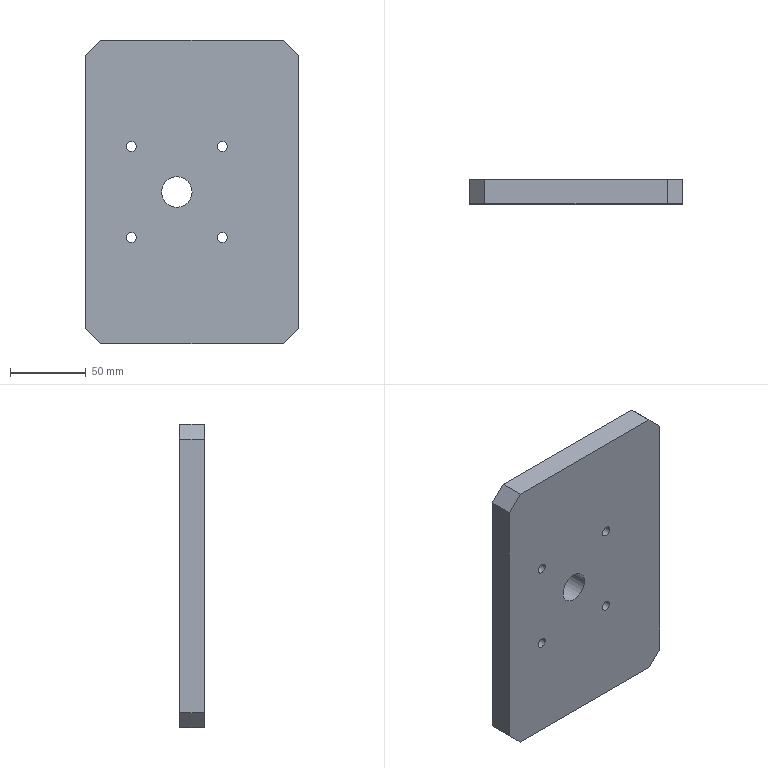Part | STEP file | M6 六角头Screw的柱形沉头Hole 2 | 1 solid | 32 faces | box 140 x 16 x 200 mm | volume 435392 mm3 | cylinder 18 | plane 14 | commonest cylinder face diameters 6.6 x8 14.55 x8 20 x2
STEP:
#1=CARTESIAN_POINT('',(-1451.463,1675.114,2786.751));
#2=VERTEX_POINT('',#1);
#3=CARTESIAN_POINT('',(-1466.013,1675.114,2786.751));
#4=VERTEX_POINT('',#3);
#5=CARTESIAN_POINT('',(-1458.738,1675.114,2786.751));
#6=DIRECTION('',(0.,1.,0.));
#7=DIRECTION('',(-1.,0.,0.));
#8=AXIS2_PLACEMENT_3D('',#5,#6,#7);
#9=CIRCLE('',#8,7.275);
#10=EDGE_CURVE('',#2,#4,#9,.T.);
#11=ORIENTED_EDGE('',*,*,#10,.F.);
#12=CARTESIAN_POINT('',(-1451.463,1679.264,2786.751));
#13=VERTEX_POINT('',#12);
#14=CARTESIAN_POINT('',(-1451.463,1679.264,2786.751));
#15=DIRECTION('',(0.,1.,0.));
#16=VECTOR('',#15,1000.);
#17=LINE('',#14,#16);
#18=EDGE_CURVE('',#2,#13,#17,.T.);
#19=ORIENTED_EDGE('',*,*,#18,.T.);
#20=CARTESIAN_POINT('',(-1466.013,1679.264,2786.751));
#21=VERTEX_POINT('',#20);
#22=CARTESIAN_POINT('',(-1458.738,1679.264,2786.751));
#23=DIRECTION('',(0.,1.,0.));
#24=DIRECTION('',(-1.,0.,0.));
#25=AXIS2_PLACEMENT_3D('',#22,#23,#24);
#26=CIRCLE('',#25,7.275);
#27=EDGE_CURVE('',#13,#21,#26,.T.);
#28=ORIENTED_EDGE('',*,*,#27,.T.);
#29=CARTESIAN_POINT('',(-1466.013,1679.264,2786.751));
#30=DIRECTION('',(0.,1.,0.));
#31=VECTOR('',#30,1000.);
#32=LINE('',#29,#31);
#33=EDGE_CURVE('',#4,#21,#32,.T.);
#34=ORIENTED_EDGE('',*,*,#33,.F.);
#35=EDGE_LOOP('',(#11,#19,#28,#34));
#36=FACE_OUTER_BOUND('',#35,.T.);
#37=CARTESIAN_POINT('',(-1458.738,1679.264,2786.751));
#38=DIRECTION('',(0.,1.,0.));
#39=DIRECTION('',(1.,0.,0.));
#40=AXIS2_PLACEMENT_3D('',#37,#38,#39);
#41=CYLINDRICAL_SURFACE('',#40,7.275);
#42=ADVANCED_FACE('',(#36),#41,.F.);
#43=CARTESIAN_POINT('',(-1455.438,1663.264,2786.751));
#44=VERTEX_POINT('',#43);
#45=CARTESIAN_POINT('',(-1462.038,1663.264,2786.751));
#46=VERTEX_POINT('',#45);
#47=CARTESIAN_POINT('',(-1458.738,1663.264,2786.751));
#48=DIRECTION('',(0.,1.,0.));
#49=DIRECTION('',(-1.,0.,0.));
#50=AXIS2_PLACEMENT_3D('',#47,#48,#49);
#51=CIRCLE('',#50,3.3);
#52=EDGE_CURVE('',#44,#46,#51,.T.);
#53=ORIENTED_EDGE('',*,*,#52,.F.);
#54=CARTESIAN_POINT('',(-1455.438,1675.114,2786.751));
#55=VERTEX_POINT('',#54);
#56=CARTESIAN_POINT('',(-1455.438,1679.264,2786.751));
#57=DIRECTION('',(0.,1.,0.));
#58=VECTOR('',#57,1000.);
#59=LINE('',#56,#58);
#60=EDGE_CURVE('',#44,#55,#59,.T.);
#61=ORIENTED_EDGE('',*,*,#60,.T.);
#62=CARTESIAN_POINT('',(-1462.038,1675.114,2786.751));
#63=VERTEX_POINT('',#62);
#64=CARTESIAN_POINT('',(-1458.738,1675.114,2786.751));
#65=DIRECTION('',(0.,1.,0.));
#66=DIRECTION('',(-1.,0.,0.));
#67=AXIS2_PLACEMENT_3D('',#64,#65,#66);
#68=CIRCLE('',#67,3.3);
#69=EDGE_CURVE('',#55,#63,#68,.T.);
#70=ORIENTED_EDGE('',*,*,#69,.T.);
#71=CARTESIAN_POINT('',(-1462.038,1679.264,2786.751));
#72=DIRECTION('',(0.,1.,0.));
#73=VECTOR('',#72,1000.);
#74=LINE('',#71,#73);
#75=EDGE_CURVE('',#46,#63,#74,.T.);
#76=ORIENTED_EDGE('',*,*,#75,.F.);
#77=EDGE_LOOP('',(#53,#61,#70,#76));
#78=FACE_OUTER_BOUND('',#77,.T.);
#79=CARTESIAN_POINT('',(-1458.738,1679.264,2786.751));
#80=DIRECTION('',(0.,1.,0.));
#81=DIRECTION('',(1.,0.,0.));
#82=AXIS2_PLACEMENT_3D('',#79,#80,#81);
#83=CYLINDRICAL_SURFACE('',#82,3.3);
#84=ADVANCED_FACE('',(#78),#83,.F.);
#85=CARTESIAN_POINT('',(-1511.463,1675.114,2846.751));
#86=VERTEX_POINT('',#85);
#87=CARTESIAN_POINT('',(-1526.013,1675.114,2846.751));
#88=VERTEX_POINT('',#87);
#89=CARTESIAN_POINT('',(-1518.738,1675.114,2846.751));
#90=DIRECTION('',(0.,1.,0.));
#91=DIRECTION('',(-1.,0.,0.));
#92=AXIS2_PLACEMENT_3D('',#89,#90,#91);
#93=CIRCLE('',#92,7.275);
#94=EDGE_CURVE('',#86,#88,#93,.T.);
#95=ORIENTED_EDGE('',*,*,#94,.F.);
#96=CARTESIAN_POINT('',(-1511.463,1679.264,2846.751));
#97=VERTEX_POINT('',#96);
#98=CARTESIAN_POINT('',(-1511.463,1679.264,2846.751));
#99=DIRECTION('',(0.,1.,0.));
#100=VECTOR('',#99,1000.);
#101=LINE('',#98,#100);
#102=EDGE_CURVE('',#86,#97,#101,.T.);
#103=ORIENTED_EDGE('',*,*,#102,.T.);
#104=CARTESIAN_POINT('',(-1526.013,1679.264,2846.751));
#105=VERTEX_POINT('',#104);
#106=CARTESIAN_POINT('',(-1518.738,1679.264,2846.751));
#107=DIRECTION('',(0.,1.,0.));
#108=DIRECTION('',(-1.,0.,0.));
#109=AXIS2_PLACEMENT_3D('',#106,#107,#108);
#110=CIRCLE('',#109,7.275);
#111=EDGE_CURVE('',#97,#105,#110,.T.);
#112=ORIENTED_EDGE('',*,*,#111,.T.);
#113=CARTESIAN_POINT('',(-1526.013,1679.264,2846.751));
#114=DIRECTION('',(0.,1.,0.));
#115=VECTOR('',#114,1000.);
#116=LINE('',#113,#115);
#117=EDGE_CURVE('',#88,#105,#116,.T.);
#118=ORIENTED_EDGE('',*,*,#117,.F.);
#119=EDGE_LOOP('',(#95,#103,#112,#118));
#120=FACE_OUTER_BOUND('',#119,.T.);
#121=CARTESIAN_POINT('',(-1518.738,1679.264,2846.751));
#122=DIRECTION('',(0.,1.,0.));
#123=DIRECTION('',(1.,0.,0.));
#124=AXIS2_PLACEMENT_3D('',#121,#122,#123);
#125=CYLINDRICAL_SURFACE('',#124,7.275);
#126=ADVANCED_FACE('',(#120),#125,.F.);
#127=CARTESIAN_POINT('',(-1515.438,1663.264,2846.751));
#128=VERTEX_POINT('',#127);
#129=CARTESIAN_POINT('',(-1522.038,1663.264,2846.751));
#130=VERTEX_POINT('',#129);
#131=CARTESIAN_POINT('',(-1518.738,1663.264,2846.751));
#132=DIRECTION('',(0.,1.,0.));
#133=DIRECTION('',(-1.,0.,0.));
#134=AXIS2_PLACEMENT_3D('',#131,#132,#133);
#135=CIRCLE('',#134,3.3);
#136=EDGE_CURVE('',#128,#130,#135,.T.);
#137=ORIENTED_EDGE('',*,*,#136,.F.);
#138=CARTESIAN_POINT('',(-1515.438,1675.114,2846.751));
#139=VERTEX_POINT('',#138);
#140=CARTESIAN_POINT('',(-1515.438,1679.264,2846.751));
#141=DIRECTION('',(0.,1.,0.));
#142=VECTOR('',#141,1000.);
#143=LINE('',#140,#142);
#144=EDGE_CURVE('',#128,#139,#143,.T.);
#145=ORIENTED_EDGE('',*,*,#144,.T.);
#146=CARTESIAN_POINT('',(-1522.038,1675.114,2846.751));
#147=VERTEX_POINT('',#146);
#148=CARTESIAN_POINT('',(-1518.738,1675.114,2846.751));
#149=DIRECTION('',(0.,1.,0.));
#150=DIRECTION('',(-1.,0.,0.));
#151=AXIS2_PLACEMENT_3D('',#148,#149,#150);
#152=CIRCLE('',#151,3.3);
#153=EDGE_CURVE('',#139,#147,#152,.T.);
#154=ORIENTED_EDGE('',*,*,#153,.T.);
#155=CARTESIAN_POINT('',(-1522.038,1679.264,2846.751));
#156=DIRECTION('',(0.,1.,0.));
#157=VECTOR('',#156,1000.);
#158=LINE('',#155,#157);
#159=EDGE_CURVE('',#130,#147,#158,.T.);
#160=ORIENTED_EDGE('',*,*,#159,.F.);
#161=EDGE_LOOP('',(#137,#145,#154,#160));
#162=FACE_OUTER_BOUND('',#161,.T.);
#163=CARTESIAN_POINT('',(-1518.738,1679.264,2846.751));
#164=DIRECTION('',(0.,1.,0.));
#165=DIRECTION('',(1.,0.,0.));
#166=AXIS2_PLACEMENT_3D('',#163,#164,#165);
#167=CYLINDRICAL_SURFACE('',#166,3.3);
#168=ADVANCED_FACE('',(#162),#167,.F.);
#169=CARTESIAN_POINT('',(-1451.463,1675.114,2846.751));
#170=VERTEX_POINT('',#169);
#171=CARTESIAN_POINT('',(-1466.013,1675.114,2846.751));
#172=VERTEX_POINT('',#171);
#173=CARTESIAN_POINT('',(-1458.738,1675.114,2846.751));
#174=DIRECTION('',(0.,1.,0.));
#175=DIRECTION('',(-1.,0.,0.));
#176=AXIS2_PLACEMENT_3D('',#173,#174,#175);
#177=CIRCLE('',#176,7.275);
#178=EDGE_CURVE('',#170,#172,#177,.T.);
#179=ORIENTED_EDGE('',*,*,#178,.F.);
#180=CARTESIAN_POINT('',(-1451.463,1679.264,2846.751));
#181=VERTEX_POINT('',#180);
#182=CARTESIAN_POINT('',(-1451.463,1679.264,2846.751));
#183=DIRECTION('',(0.,1.,0.));
#184=VECTOR('',#183,1000.);
#185=LINE('',#182,#184);
#186=EDGE_CURVE('',#170,#181,#185,.T.);
#187=ORIENTED_EDGE('',*,*,#186,.T.);
#188=CARTESIAN_POINT('',(-1466.013,1679.264,2846.751));
#189=VERTEX_POINT('',#188);
#190=CARTESIAN_POINT('',(-1458.738,1679.264,2846.751));
#191=DIRECTION('',(0.,1.,0.));
#192=DIRECTION('',(-1.,0.,0.));
#193=AXIS2_PLACEMENT_3D('',#190,#191,#192);
#194=CIRCLE('',#193,7.275);
#195=EDGE_CURVE('',#181,#189,#194,.T.);
#196=ORIENTED_EDGE('',*,*,#195,.T.);
#197=CARTESIAN_POINT('',(-1466.013,1679.264,2846.751));
#198=DIRECTION('',(0.,1.,0.));
#199=VECTOR('',#198,1000.);
#200=LINE('',#197,#199);
#201=EDGE_CURVE('',#172,#189,#200,.T.);
#202=ORIENTED_EDGE('',*,*,#201,.F.);
#203=EDGE_LOOP('',(#179,#187,#196,#202));
#204=FACE_OUTER_BOUND('',#203,.T.);
#205=CARTESIAN_POINT('',(-1458.738,1679.264,2846.751));
#206=DIRECTION('',(0.,1.,0.));
#207=DIRECTION('',(1.,0.,0.));
#208=AXIS2_PLACEMENT_3D('',#205,#206,#207);
#209=CYLINDRICAL_SURFACE('',#208,7.275);
#210=ADVANCED_FACE('',(#204),#209,.F.);
#211=CARTESIAN_POINT('',(-1455.438,1663.264,2846.751));
#212=VERTEX_POINT('',#211);
#213=CARTESIAN_POINT('',(-1462.038,1663.264,2846.751));
#214=VERTEX_POINT('',#213);
#215=CARTESIAN_POINT('',(-1458.738,1663.264,2846.751));
#216=DIRECTION('',(0.,1.,0.));
#217=DIRECTION('',(-1.,0.,0.));
#218=AXIS2_PLACEMENT_3D('',#215,#216,#217);
#219=CIRCLE('',#218,3.3);
#220=EDGE_CURVE('',#212,#214,#219,.T.);
#221=ORIENTED_EDGE('',*,*,#220,.F.);
#222=CARTESIAN_POINT('',(-1455.438,1675.114,2846.751));
#223=VERTEX_POINT('',#222);
#224=CARTESIAN_POINT('',(-1455.438,1679.264,2846.751));
#225=DIRECTION('',(0.,1.,0.));
#226=VECTOR('',#225,1000.);
#227=LINE('',#224,#226);
#228=EDGE_CURVE('',#212,#223,#227,.T.);
#229=ORIENTED_EDGE('',*,*,#228,.T.);
#230=CARTESIAN_POINT('',(-1462.038,1675.114,2846.751));
#231=VERTEX_POINT('',#230);
#232=CARTESIAN_POINT('',(-1458.738,1675.114,2846.751));
#233=DIRECTION('',(0.,1.,0.));
#234=DIRECTION('',(-1.,0.,0.));
#235=AXIS2_PLACEMENT_3D('',#232,#233,#234);
#236=CIRCLE('',#235,3.3);
#237=EDGE_CURVE('',#223,#231,#236,.T.);
#238=ORIENTED_EDGE('',*,*,#237,.T.);
#239=CARTESIAN_POINT('',(-1462.038,1679.264,2846.751));
#240=DIRECTION('',(0.,1.,0.));
#241=VECTOR('',#240,1000.);
#242=LINE('',#239,#241);
#243=EDGE_CURVE('',#214,#231,#242,.T.);
#244=ORIENTED_EDGE('',*,*,#243,.F.);
#245=EDGE_LOOP('',(#221,#229,#238,#244));
#246=FACE_OUTER_BOUND('',#245,.T.);
#247=CARTESIAN_POINT('',(-1458.738,1679.264,2846.751));
#248=DIRECTION('',(0.,1.,0.));
#249=DIRECTION('',(1.,0.,0.));
#250=AXIS2_PLACEMENT_3D('',#247,#248,#249);
#251=CYLINDRICAL_SURFACE('',#250,3.3);
#252=ADVANCED_FACE('',(#246),#251,.F.);
#253=CARTESIAN_POINT('',(-1511.463,1675.114,2786.751));
#254=VERTEX_POINT('',#253);
#255=CARTESIAN_POINT('',(-1526.013,1675.114,2786.751));
#256=VERTEX_POINT('',#255);
#257=CARTESIAN_POINT('',(-1518.738,1675.114,2786.751));
#258=DIRECTION('',(0.,1.,0.));
#259=DIRECTION('',(-1.,0.,0.));
#260=AXIS2_PLACEMENT_3D('',#257,#258,#259);
#261=CIRCLE('',#260,7.275);
#262=EDGE_CURVE('',#254,#256,#261,.T.);
#263=ORIENTED_EDGE('',*,*,#262,.F.);
#264=CARTESIAN_POINT('',(-1511.463,1679.264,2786.751));
#265=VERTEX_POINT('',#264);
#266=CARTESIAN_POINT('',(-1511.463,1679.264,2786.751));
#267=DIRECTION('',(0.,1.,0.));
#268=VECTOR('',#267,1000.);
#269=LINE('',#266,#268);
#270=EDGE_CURVE('',#254,#265,#269,.T.);
#271=ORIENTED_EDGE('',*,*,#270,.T.);
#272=CARTESIAN_POINT('',(-1526.013,1679.264,2786.751));
#273=VERTEX_POINT('',#272);
#274=CARTESIAN_POINT('',(-1518.738,1679.264,2786.751));
#275=DIRECTION('',(0.,1.,0.));
#276=DIRECTION('',(-1.,0.,0.));
#277=AXIS2_PLACEMENT_3D('',#274,#275,#276);
#278=CIRCLE('',#277,7.275);
#279=EDGE_CURVE('',#265,#273,#278,.T.);
#280=ORIENTED_EDGE('',*,*,#279,.T.);
#281=CARTESIAN_POINT('',(-1526.013,1679.264,2786.751));
#282=DIRECTION('',(0.,1.,0.));
#283=VECTOR('',#282,1000.);
#284=LINE('',#281,#283);
#285=EDGE_CURVE('',#256,#273,#284,.T.);
#286=ORIENTED_EDGE('',*,*,#285,.F.);
#287=EDGE_LOOP('',(#263,#271,#280,#286));
#288=FACE_OUTER_BOUND('',#287,.T.);
#289=CARTESIAN_POINT('',(-1518.738,1679.264,2786.751));
#290=DIRECTION('',(0.,1.,0.));
#291=DIRECTION('',(1.,0.,0.));
#292=AXIS2_PLACEMENT_3D('',#289,#290,#291);
#293=CYLINDRICAL_SURFACE('',#292,7.275);
#294=ADVANCED_FACE('',(#288),#293,.F.);
#295=CARTESIAN_POINT('',(-1515.438,1663.264,2786.751));
#296=VERTEX_POINT('',#295);
#297=CARTESIAN_POINT('',(-1522.038,1663.264,2786.751));
#298=VERTEX_POINT('',#297);
#299=CARTESIAN_POINT('',(-1518.738,1663.264,2786.751));
#300=DIRECTION('',(0.,1.,0.));
#301=DIRECTION('',(-1.,0.,0.));
#302=AXIS2_PLACEMENT_3D('',#299,#300,#301);
#303=CIRCLE('',#302,3.3);
#304=EDGE_CURVE('',#296,#298,#303,.T.);
#305=ORIENTED_EDGE('',*,*,#304,.F.);
#306=CARTESIAN_POINT('',(-1515.438,1675.114,2786.751));
#307=VERTEX_POINT('',#306);
#308=CARTESIAN_POINT('',(-1515.438,1679.264,2786.751));
#309=DIRECTION('',(0.,1.,0.));
#310=VECTOR('',#309,1000.);
#311=LINE('',#308,#310);
#312=EDGE_CURVE('',#296,#307,#311,.T.);
#313=ORIENTED_EDGE('',*,*,#312,.T.);
#314=CARTESIAN_POINT('',(-1522.038,1675.114,2786.751));
#315=VERTEX_POINT('',#314);
#316=CARTESIAN_POINT('',(-1518.738,1675.114,2786.751));
#317=DIRECTION('',(0.,1.,0.));
#318=DIRECTION('',(-1.,0.,0.));
#319=AXIS2_PLACEMENT_3D('',#316,#317,#318);
#320=CIRCLE('',#319,3.3);
#321=EDGE_CURVE('',#307,#315,#320,.T.);
#322=ORIENTED_EDGE('',*,*,#321,.T.);
#323=CARTESIAN_POINT('',(-1522.038,1679.264,2786.751));
#324=DIRECTION('',(0.,1.,0.));
#325=VECTOR('',#324,1000.);
#326=LINE('',#323,#325);
#327=EDGE_CURVE('',#298,#315,#326,.T.);
#328=ORIENTED_EDGE('',*,*,#327,.F.);
#329=EDGE_LOOP('',(#305,#313,#322,#328));
#330=FACE_OUTER_BOUND('',#329,.T.);
#331=CARTESIAN_POINT('',(-1518.738,1679.264,2786.751));
#332=DIRECTION('',(0.,1.,0.));
#333=DIRECTION('',(1.,0.,0.));
#334=AXIS2_PLACEMENT_3D('',#331,#332,#333);
#335=CYLINDRICAL_SURFACE('',#334,3.3);
#336=ADVANCED_FACE('',(#330),#335,.F.);
#337=CARTESIAN_POINT('',(-1478.738,1663.264,2816.751));
#338=VERTEX_POINT('',#337);
#339=CARTESIAN_POINT('',(-1498.738,1663.264,2816.751));
#340=VERTEX_POINT('',#339);
#341=CARTESIAN_POINT('',(-1488.738,1663.264,2816.751));
#342=DIRECTION('',(0.,1.,0.));
#343=DIRECTION('',(-1.,0.,0.));
#344=AXIS2_PLACEMENT_3D('',#341,#342,#343);
#345=CIRCLE('',#344,10.);
#346=EDGE_CURVE('',#338,#340,#345,.T.);
#347=ORIENTED_EDGE('',*,*,#346,.F.);
#348=CARTESIAN_POINT('',(-1478.738,1679.264,2816.751));
#349=VERTEX_POINT('',#348);
#350=CARTESIAN_POINT('',(-1478.738,1573.264,2816.751));
#351=DIRECTION('',(0.,1.,0.));
#352=VECTOR('',#351,1000.);
#353=LINE('',#350,#352);
#354=EDGE_CURVE('',#338,#349,#353,.T.);
#355=ORIENTED_EDGE('',*,*,#354,.T.);
#356=CARTESIAN_POINT('',(-1498.738,1679.264,2816.751));
#357=VERTEX_POINT('',#356);
#358=CARTESIAN_POINT('',(-1488.738,1679.264,2816.751));
#359=DIRECTION('',(0.,1.,0.));
#360=DIRECTION('',(-1.,0.,0.));
#361=AXIS2_PLACEMENT_3D('',#358,#359,#360);
#362=CIRCLE('',#361,10.);
#363=EDGE_CURVE('',#349,#357,#362,.T.);
#364=ORIENTED_EDGE('',*,*,#363,.T.);
#365=CARTESIAN_POINT('',(-1498.738,1573.264,2816.751));
#366=DIRECTION('',(0.,1.,0.));
#367=VECTOR('',#366,1000.);
#368=LINE('',#365,#367);
#369=EDGE_CURVE('',#340,#357,#368,.T.);
#370=ORIENTED_EDGE('',*,*,#369,.F.);
#371=EDGE_LOOP('',(#347,#355,#364,#370));
#372=FACE_OUTER_BOUND('',#371,.T.);
#373=CARTESIAN_POINT('',(-1488.738,1573.264,2816.751));
#374=DIRECTION('',(0.,1.,0.));
#375=DIRECTION('',(1.,0.,0.));
#376=AXIS2_PLACEMENT_3D('',#373,#374,#375);
#377=CYLINDRICAL_SURFACE('',#376,10.);
#378=ADVANCED_FACE('',(#372),#377,.F.);
#379=CARTESIAN_POINT('',(-1538.738,1663.264,2916.751));
#380=VERTEX_POINT('',#379);
#381=CARTESIAN_POINT('',(-1418.738,1663.264,2916.751));
#382=VERTEX_POINT('',#381);
#383=CARTESIAN_POINT('',(-1408.738,1663.264,2916.751));
#384=DIRECTION('',(1.,0.,0.));
#385=VECTOR('',#384,1000.);
#386=LINE('',#383,#385);
#387=EDGE_CURVE('',#380,#382,#386,.T.);
#388=ORIENTED_EDGE('',*,*,#387,.T.);
#389=CARTESIAN_POINT('',(-1418.738,1679.264,2916.751));
#390=VERTEX_POINT('',#389);
#391=CARTESIAN_POINT('',(-1418.738,1679.264,2916.751));
#392=DIRECTION('',(0.,1.,0.));
#393=VECTOR('',#392,1000.);
#394=LINE('',#391,#393);
#395=EDGE_CURVE('',#382,#390,#394,.T.);
#396=ORIENTED_EDGE('',*,*,#395,.T.);
#397=CARTESIAN_POINT('',(-1538.738,1679.264,2916.751));
#398=VERTEX_POINT('',#397);
#399=CARTESIAN_POINT('',(-1408.738,1679.264,2916.751));
#400=DIRECTION('',(1.,0.,0.));
#401=VECTOR('',#400,1000.);
#402=LINE('',#399,#401);
#403=EDGE_CURVE('',#398,#390,#402,.T.);
#404=ORIENTED_EDGE('',*,*,#403,.F.);
#405=CARTESIAN_POINT('',(-1538.738,1679.264,2916.751));
#406=DIRECTION('',(0.,-1.,0.));
#407=VECTOR('',#406,1000.);
#408=LINE('',#405,#407);
#409=EDGE_CURVE('',#398,#380,#408,.T.);
#410=ORIENTED_EDGE('',*,*,#409,.T.);
#411=EDGE_LOOP('',(#388,#396,#404,#410));
#412=FACE_OUTER_BOUND('',#411,.T.);
#413=CARTESIAN_POINT('',(-1408.738,1679.264,2916.751));
#414=DIRECTION('',(0.,0.,-1.));
#415=DIRECTION('',(1.,0.,0.));
#416=AXIS2_PLACEMENT_3D('',#413,#414,#415);
#417=PLANE('',#416);
#418=ADVANCED_FACE('',(#412),#417,.F.);
#419=CARTESIAN_POINT('',(-1408.738,1679.264,2906.751));
#420=VERTEX_POINT('',#419);
#421=CARTESIAN_POINT('',(-1408.738,1679.264,2726.751));
#422=VERTEX_POINT('',#421);
#423=CARTESIAN_POINT('',(-1408.738,1679.264,2716.751));
#424=DIRECTION('',(0.,0.,-1.));
#425=VECTOR('',#424,1000.);
#426=LINE('',#423,#425);
#427=EDGE_CURVE('',#420,#422,#426,.T.);
#428=ORIENTED_EDGE('',*,*,#427,.F.);
#429=CARTESIAN_POINT('',(-1408.738,1663.264,2906.751));
#430=VERTEX_POINT('',#429);
#431=CARTESIAN_POINT('',(-1408.738,1679.264,2906.751));
#432=DIRECTION('',(0.,-1.,0.));
#433=VECTOR('',#432,1000.);
#434=LINE('',#431,#433);
#435=EDGE_CURVE('',#420,#430,#434,.T.);
#436=ORIENTED_EDGE('',*,*,#435,.T.);
#437=CARTESIAN_POINT('',(-1408.738,1663.264,2726.751));
#438=VERTEX_POINT('',#437);
#439=CARTESIAN_POINT('',(-1408.738,1663.264,2716.751));
#440=DIRECTION('',(0.,0.,-1.));
#441=VECTOR('',#440,1000.);
#442=LINE('',#439,#441);
#443=EDGE_CURVE('',#430,#438,#442,.T.);
#444=ORIENTED_EDGE('',*,*,#443,.T.);
#445=CARTESIAN_POINT('',(-1408.738,1679.264,2726.751));
#446=DIRECTION('',(0.,1.,0.));
#447=VECTOR('',#446,1000.);
#448=LINE('',#445,#447);
#449=EDGE_CURVE('',#438,#422,#448,.T.);
#450=ORIENTED_EDGE('',*,*,#449,.T.);
#451=EDGE_LOOP('',(#428,#436,#444,#450));
#452=FACE_OUTER_BOUND('',#451,.T.);
#453=CARTESIAN_POINT('',(-1408.738,1679.264,2716.751));
#454=DIRECTION('',(-1.,0.,0.));
#455=DIRECTION('',(0.,0.,-1.));
#456=AXIS2_PLACEMENT_3D('',#453,#454,#455);
#457=PLANE('',#456);
#458=ADVANCED_FACE('',(#452),#457,.F.);
#459=CARTESIAN_POINT('',(-1418.738,1663.264,2716.751));
#460=VERTEX_POINT('',#459);
#461=CARTESIAN_POINT('',(-1538.738,1663.264,2716.751));
#462=VERTEX_POINT('',#461);
#463=CARTESIAN_POINT('',(-1408.738,1663.264,2716.751));
#464=DIRECTION('',(-1.,0.,0.));
#465=VECTOR('',#464,1000.);
#466=LINE('',#463,#465);
#467=EDGE_CURVE('',#460,#462,#466,.T.);
#468=ORIENTED_EDGE('',*,*,#467,.T.);
#469=CARTESIAN_POINT('',(-1538.738,1679.264,2716.751));
#470=VERTEX_POINT('',#469);
#471=CARTESIAN_POINT('',(-1538.738,1679.264,2716.751));
#472=DIRECTION('',(0.,1.,0.));
#473=VECTOR('',#472,1000.);
#474=LINE('',#471,#473);
#475=EDGE_CURVE('',#462,#470,#474,.T.);
#476=ORIENTED_EDGE('',*,*,#475,.T.);
#477=CARTESIAN_POINT('',(-1418.738,1679.264,2716.751));
#478=VERTEX_POINT('',#477);
#479=CARTESIAN_POINT('',(-1408.738,1679.264,2716.751));
#480=DIRECTION('',(-1.,0.,0.));
#481=VECTOR('',#480,1000.);
#482=LINE('',#479,#481);
#483=EDGE_CURVE('',#478,#470,#482,.T.);
#484=ORIENTED_EDGE('',*,*,#483,.F.);
#485=CARTESIAN_POINT('',(-1418.738,1679.264,2716.751));
#486=DIRECTION('',(0.,-1.,0.));
#487=VECTOR('',#486,1000.);
#488=LINE('',#485,#487);
#489=EDGE_CURVE('',#478,#460,#488,.T.);
#490=ORIENTED_EDGE('',*,*,#489,.T.);
#491=EDGE_LOOP('',(#468,#476,#484,#490));
#492=FACE_OUTER_BOUND('',#491,.T.);
#493=CARTESIAN_POINT('',(-1408.738,1679.264,2716.751));
#494=DIRECTION('',(0.,0.,1.));
#495=DIRECTION('',(-1.,0.,0.));
#496=AXIS2_PLACEMENT_3D('',#493,#494,#495);
#497=PLANE('',#496);
#498=ADVANCED_FACE('',(#492),#497,.F.);
#499=CARTESIAN_POINT('',(-1548.738,1663.264,2726.751));
#500=VERTEX_POINT('',#499);
#501=CARTESIAN_POINT('',(-1548.738,1663.264,2906.751));
#502=VERTEX_POINT('',#501);
#503=CARTESIAN_POINT('',(-1548.738,1663.264,2716.751));
#504=DIRECTION('',(0.,0.,1.));
#505=VECTOR('',#504,1000.);
#506=LINE('',#503,#505);
#507=EDGE_CURVE('',#500,#502,#506,.T.);
#508=ORIENTED_EDGE('',*,*,#507,.T.);
#509=CARTESIAN_POINT('',(-1548.738,1679.264,2906.751));
#510=VERTEX_POINT('',#509);
#511=CARTESIAN_POINT('',(-1548.738,1679.264,2906.751));
#512=DIRECTION('',(0.,1.,0.));
#513=VECTOR('',#512,1000.);
#514=LINE('',#511,#513);
#515=EDGE_CURVE('',#502,#510,#514,.T.);
#516=ORIENTED_EDGE('',*,*,#515,.T.);
#517=CARTESIAN_POINT('',(-1548.738,1679.264,2726.751));
#518=VERTEX_POINT('',#517);
#519=CARTESIAN_POINT('',(-1548.738,1679.264,2716.751));
#520=DIRECTION('',(0.,0.,1.));
#521=VECTOR('',#520,1000.);
#522=LINE('',#519,#521);
#523=EDGE_CURVE('',#518,#510,#522,.T.);
#524=ORIENTED_EDGE('',*,*,#523,.F.);
#525=CARTESIAN_POINT('',(-1548.738,1679.264,2726.751));
#526=DIRECTION('',(0.,-1.,0.));
#527=VECTOR('',#526,1000.);
#528=LINE('',#525,#527);
#529=EDGE_CURVE('',#518,#500,#528,.T.);
#530=ORIENTED_EDGE('',*,*,#529,.T.);
#531=EDGE_LOOP('',(#508,#516,#524,#530));
#532=FACE_OUTER_BOUND('',#531,.T.);
#533=CARTESIAN_POINT('',(-1548.738,1679.264,2716.751));
#534=DIRECTION('',(1.,0.,0.));
#535=DIRECTION('',(0.,0.,1.));
#536=AXIS2_PLACEMENT_3D('',#533,#534,#535);
#537=PLANE('',#536);
#538=ADVANCED_FACE('',(#532),#537,.F.);
#539=CARTESIAN_POINT('',(-1458.738,1679.264,2786.751));
#540=DIRECTION('',(0.,1.,0.));
#541=DIRECTION('',(-1.,0.,0.));
#542=AXIS2_PLACEMENT_3D('',#539,#540,#541);
#543=CIRCLE('',#542,7.275);
#544=EDGE_CURVE('',#21,#13,#543,.T.);
#545=ORIENTED_EDGE('',*,*,#544,.F.);
#546=ORIENTED_EDGE('',*,*,#27,.F.);
#547=EDGE_LOOP('',(#545,#546));
#548=FACE_BOUND('',#547,.T.);
#549=CARTESIAN_POINT('',(-1518.738,1679.264,2846.751));
#550=DIRECTION('',(0.,1.,0.));
#551=DIRECTION('',(-1.,0.,0.));
#552=AXIS2_PLACEMENT_3D('',#549,#550,#551);
#553=CIRCLE('',#552,7.275);
#554=EDGE_CURVE('',#105,#97,#553,.T.);
#555=ORIENTED_EDGE('',*,*,#554,.F.);
#556=ORIENTED_EDGE('',*,*,#111,.F.);
#557=EDGE_LOOP('',(#555,#556));
#558=FACE_BOUND('',#557,.T.);
#559=CARTESIAN_POINT('',(-1458.738,1679.264,2846.751));
#560=DIRECTION('',(0.,1.,0.));
#561=DIRECTION('',(-1.,0.,0.));
#562=AXIS2_PLACEMENT_3D('',#559,#560,#561);
#563=CIRCLE('',#562,7.275);
#564=EDGE_CURVE('',#189,#181,#563,.T.);
#565=ORIENTED_EDGE('',*,*,#564,.F.);
#566=ORIENTED_EDGE('',*,*,#195,.F.);
#567=EDGE_LOOP('',(#565,#566));
#568=FACE_BOUND('',#567,.T.);
#569=CARTESIAN_POINT('',(-1518.738,1679.264,2786.751));
#570=DIRECTION('',(0.,1.,0.));
#571=DIRECTION('',(-1.,0.,0.));
#572=AXIS2_PLACEMENT_3D('',#569,#570,#571);
#573=CIRCLE('',#572,7.275);
#574=EDGE_CURVE('',#273,#265,#573,.T.);
#575=ORIENTED_EDGE('',*,*,#574,.F.);
#576=ORIENTED_EDGE('',*,*,#279,.F.);
#577=EDGE_LOOP('',(#575,#576));
#578=FACE_BOUND('',#577,.T.);
#579=CARTESIAN_POINT('',(-1488.738,1679.264,2816.751));
#580=DIRECTION('',(0.,1.,0.));
#581=DIRECTION('',(-1.,0.,0.));
#582=AXIS2_PLACEMENT_3D('',#579,#580,#581);
#583=CIRCLE('',#582,10.);
#584=EDGE_CURVE('',#357,#349,#583,.T.);
#585=ORIENTED_EDGE('',*,*,#584,.F.);
#586=ORIENTED_EDGE('',*,*,#363,.F.);
#587=EDGE_LOOP('',(#585,#586));
#588=FACE_BOUND('',#587,.T.);
#589=ORIENTED_EDGE('',*,*,#403,.T.);
#590=CARTESIAN_POINT('',(-1398.738,1679.264,2896.751));
#591=DIRECTION('',(0.7071,0.,-0.7071));
#592=VECTOR('',#591,1000.);
#593=LINE('',#590,#592);
#594=EDGE_CURVE('',#390,#420,#593,.T.);
#595=ORIENTED_EDGE('',*,*,#594,.T.);
#596=ORIENTED_EDGE('',*,*,#427,.T.);
#597=CARTESIAN_POINT('',(-1398.738,1679.264,2736.751));
#598=DIRECTION('',(-0.7071,0.,-0.7071));
#599=VECTOR('',#598,1000.);
#600=LINE('',#597,#599);
#601=EDGE_CURVE('',#422,#478,#600,.T.);
#602=ORIENTED_EDGE('',*,*,#601,.T.);
#603=ORIENTED_EDGE('',*,*,#483,.T.);
#604=CARTESIAN_POINT('',(-1558.738,1679.264,2736.751));
#605=DIRECTION('',(-0.7071,0.,0.7071));
#606=VECTOR('',#605,1000.);
#607=LINE('',#604,#606);
#608=EDGE_CURVE('',#470,#518,#607,.T.);
#609=ORIENTED_EDGE('',*,*,#608,.T.);
#610=ORIENTED_EDGE('',*,*,#523,.T.);
#611=CARTESIAN_POINT('',(-1558.738,1679.264,2896.751));
#612=DIRECTION('',(0.7071,0.,0.7071));
#613=VECTOR('',#612,1000.);
#614=LINE('',#611,#613);
#615=EDGE_CURVE('',#510,#398,#614,.T.);
#616=ORIENTED_EDGE('',*,*,#615,.T.);
#617=EDGE_LOOP('',(#589,#595,#596,#602,#603,#609,#610,#616));
#618=FACE_OUTER_BOUND('',#617,.T.);
#619=CARTESIAN_POINT('',(-1478.738,1679.264,2816.751));
#620=DIRECTION('',(0.,1.,0.));
#621=DIRECTION('',(1.,0.,0.));
#622=AXIS2_PLACEMENT_3D('',#619,#620,#621);
#623=PLANE('',#622);
#624=ADVANCED_FACE('',(#548,#558,#568,#578,#588,#618),#623,.T.);
#625=CARTESIAN_POINT('',(-1458.738,1663.264,2786.751));
#626=DIRECTION('',(0.,1.,0.));
#627=DIRECTION('',(-1.,0.,0.));
#628=AXIS2_PLACEMENT_3D('',#625,#626,#627);
#629=CIRCLE('',#628,3.3);
#630=EDGE_CURVE('',#46,#44,#629,.T.);
#631=ORIENTED_EDGE('',*,*,#630,.T.);
#632=ORIENTED_EDGE('',*,*,#52,.T.);
#633=EDGE_LOOP('',(#631,#632));
#634=FACE_BOUND('',#633,.T.);
#635=CARTESIAN_POINT('',(-1518.738,1663.264,2846.751));
#636=DIRECTION('',(0.,1.,0.));
#637=DIRECTION('',(-1.,0.,0.));
#638=AXIS2_PLACEMENT_3D('',#635,#636,#637);
#639=CIRCLE('',#638,3.3);
#640=EDGE_CURVE('',#130,#128,#639,.T.);
#641=ORIENTED_EDGE('',*,*,#640,.T.);
#642=ORIENTED_EDGE('',*,*,#136,.T.);
#643=EDGE_LOOP('',(#641,#642));
#644=FACE_BOUND('',#643,.T.);
#645=CARTESIAN_POINT('',(-1458.738,1663.264,2846.751));
#646=DIRECTION('',(0.,1.,0.));
#647=DIRECTION('',(-1.,0.,0.));
#648=AXIS2_PLACEMENT_3D('',#645,#646,#647);
#649=CIRCLE('',#648,3.3);
#650=EDGE_CURVE('',#214,#212,#649,.T.);
#651=ORIENTED_EDGE('',*,*,#650,.T.);
#652=ORIENTED_EDGE('',*,*,#220,.T.);
#653=EDGE_LOOP('',(#651,#652));
#654=FACE_BOUND('',#653,.T.);
#655=CARTESIAN_POINT('',(-1518.738,1663.264,2786.751));
#656=DIRECTION('',(0.,1.,0.));
#657=DIRECTION('',(-1.,0.,0.));
#658=AXIS2_PLACEMENT_3D('',#655,#656,#657);
#659=CIRCLE('',#658,3.3);
#660=EDGE_CURVE('',#298,#296,#659,.T.);
#661=ORIENTED_EDGE('',*,*,#660,.T.);
#662=ORIENTED_EDGE('',*,*,#304,.T.);
#663=EDGE_LOOP('',(#661,#662));
#664=FACE_BOUND('',#663,.T.);
#665=CARTESIAN_POINT('',(-1488.738,1663.264,2816.751));
#666=DIRECTION('',(0.,1.,0.));
#667=DIRECTION('',(-1.,0.,0.));
#668=AXIS2_PLACEMENT_3D('',#665,#666,#667);
#669=CIRCLE('',#668,10.);
#670=EDGE_CURVE('',#340,#338,#669,.T.);
#671=ORIENTED_EDGE('',*,*,#670,.T.);
#672=ORIENTED_EDGE('',*,*,#346,.T.);
#673=EDGE_LOOP('',(#671,#672));
#674=FACE_BOUND('',#673,.T.);
#675=ORIENTED_EDGE('',*,*,#443,.F.);
#676=CARTESIAN_POINT('',(-1408.738,1663.264,2906.751));
#677=DIRECTION('',(-0.7071,0.,0.7071));
#678=VECTOR('',#677,1000.);
#679=LINE('',#676,#678);
#680=EDGE_CURVE('',#430,#382,#679,.T.);
#681=ORIENTED_EDGE('',*,*,#680,.T.);
#682=ORIENTED_EDGE('',*,*,#387,.F.);
#683=CARTESIAN_POINT('',(-1538.738,1663.264,2916.751));
#684=DIRECTION('',(-0.7071,0.,-0.7071));
#685=VECTOR('',#684,1000.);
#686=LINE('',#683,#685);
#687=EDGE_CURVE('',#380,#502,#686,.T.);
#688=ORIENTED_EDGE('',*,*,#687,.T.);
#689=ORIENTED_EDGE('',*,*,#507,.F.);
#690=CARTESIAN_POINT('',(-1548.738,1663.264,2726.751));
#691=DIRECTION('',(0.7071,0.,-0.7071));
#692=VECTOR('',#691,1000.);
#693=LINE('',#690,#692);
#694=EDGE_CURVE('',#500,#462,#693,.T.);
#695=ORIENTED_EDGE('',*,*,#694,.T.);
#696=ORIENTED_EDGE('',*,*,#467,.F.);
#697=CARTESIAN_POINT('',(-1418.738,1663.264,2716.751));
#698=DIRECTION('',(0.7071,0.,0.7071));
#699=VECTOR('',#698,1000.);
#700=LINE('',#697,#699);
#701=EDGE_CURVE('',#460,#438,#700,.T.);
#702=ORIENTED_EDGE('',*,*,#701,.T.);
#703=EDGE_LOOP('',(#675,#681,#682,#688,#689,#695,#696,#702));
#704=FACE_OUTER_BOUND('',#703,.T.);
#705=CARTESIAN_POINT('',(-1478.738,1663.264,2816.751));
#706=DIRECTION('',(0.,1.,0.));
#707=DIRECTION('',(1.,0.,0.));
#708=AXIS2_PLACEMENT_3D('',#705,#706,#707);
#709=PLANE('',#708);
#710=ADVANCED_FACE('',(#634,#644,#654,#664,#674,#704),#709,.F.);
#711=ORIENTED_EDGE('',*,*,#594,.F.);
#712=ORIENTED_EDGE('',*,*,#395,.F.);
#713=ORIENTED_EDGE('',*,*,#680,.F.);
#714=ORIENTED_EDGE('',*,*,#435,.F.);
#715=EDGE_LOOP('',(#711,#712,#713,#714));
#716=FACE_OUTER_BOUND('',#715,.T.);
#717=CARTESIAN_POINT('',(-1408.738,1679.264,2906.751));
#718=DIRECTION('',(-0.7071,0.,-0.7071));
#719=DIRECTION('',(0.,1.,0.));
#720=AXIS2_PLACEMENT_3D('',#717,#718,#719);
#721=PLANE('',#720);
#722=ADVANCED_FACE('',(#716),#721,.F.);
#723=ORIENTED_EDGE('',*,*,#615,.F.);
#724=ORIENTED_EDGE('',*,*,#515,.F.);
#725=ORIENTED_EDGE('',*,*,#687,.F.);
#726=ORIENTED_EDGE('',*,*,#409,.F.);
#727=EDGE_LOOP('',(#723,#724,#725,#726));
#728=FACE_OUTER_BOUND('',#727,.T.);
#729=CARTESIAN_POINT('',(-1538.738,1679.264,2916.751));
#730=DIRECTION('',(0.7071,0.,-0.7071));
#731=DIRECTION('',(0.,1.,0.));
#732=AXIS2_PLACEMENT_3D('',#729,#730,#731);
#733=PLANE('',#732);
#734=ADVANCED_FACE('',(#728),#733,.F.);
#735=ORIENTED_EDGE('',*,*,#608,.F.);
#736=ORIENTED_EDGE('',*,*,#475,.F.);
#737=ORIENTED_EDGE('',*,*,#694,.F.);
#738=ORIENTED_EDGE('',*,*,#529,.F.);
#739=EDGE_LOOP('',(#735,#736,#737,#738));
#740=FACE_OUTER_BOUND('',#739,.T.);
#741=CARTESIAN_POINT('',(-1548.738,1679.264,2726.751));
#742=DIRECTION('',(0.7071,0.,0.7071));
#743=DIRECTION('',(0.,1.,0.));
#744=AXIS2_PLACEMENT_3D('',#741,#742,#743);
#745=PLANE('',#744);
#746=ADVANCED_FACE('',(#740),#745,.F.);
#747=ORIENTED_EDGE('',*,*,#601,.F.);
#748=ORIENTED_EDGE('',*,*,#449,.F.);
#749=ORIENTED_EDGE('',*,*,#701,.F.);
#750=ORIENTED_EDGE('',*,*,#489,.F.);
#751=EDGE_LOOP('',(#747,#748,#749,#750));
#752=FACE_OUTER_BOUND('',#751,.T.);
#753=CARTESIAN_POINT('',(-1418.738,1679.264,2716.751));
#754=DIRECTION('',(-0.7071,0.,0.7071));
#755=DIRECTION('',(0.,1.,0.));
#756=AXIS2_PLACEMENT_3D('',#753,#754,#755);
#757=PLANE('',#756);
#758=ADVANCED_FACE('',(#752),#757,.F.);
#759=ORIENTED_EDGE('',*,*,#354,.F.);
#760=ORIENTED_EDGE('',*,*,#670,.F.);
#761=ORIENTED_EDGE('',*,*,#369,.T.);
#762=ORIENTED_EDGE('',*,*,#584,.T.);
#763=EDGE_LOOP('',(#759,#760,#761,#762));
#764=FACE_OUTER_BOUND('',#763,.T.);
#765=CARTESIAN_POINT('',(-1488.738,1573.264,2816.751));
#766=DIRECTION('',(0.,1.,0.));
#767=DIRECTION('',(1.,0.,0.));
#768=AXIS2_PLACEMENT_3D('',#765,#766,#767);
#769=CYLINDRICAL_SURFACE('',#768,10.);
#770=ADVANCED_FACE('',(#764),#769,.F.);
#771=ORIENTED_EDGE('',*,*,#312,.F.);
#772=ORIENTED_EDGE('',*,*,#660,.F.);
#773=ORIENTED_EDGE('',*,*,#327,.T.);
#774=CARTESIAN_POINT('',(-1518.738,1675.114,2786.751));
#775=DIRECTION('',(0.,1.,0.));
#776=DIRECTION('',(-1.,0.,0.));
#777=AXIS2_PLACEMENT_3D('',#774,#775,#776);
#778=CIRCLE('',#777,3.3);
#779=EDGE_CURVE('',#315,#307,#778,.T.);
#780=ORIENTED_EDGE('',*,*,#779,.T.);
#781=EDGE_LOOP('',(#771,#772,#773,#780));
#782=FACE_OUTER_BOUND('',#781,.T.);
#783=CARTESIAN_POINT('',(-1518.738,1679.264,2786.751));
#784=DIRECTION('',(0.,1.,0.));
#785=DIRECTION('',(1.,0.,0.));
#786=AXIS2_PLACEMENT_3D('',#783,#784,#785);
#787=CYLINDRICAL_SURFACE('',#786,3.3);
#788=ADVANCED_FACE('',(#782),#787,.F.);
#789=ORIENTED_EDGE('',*,*,#779,.F.);
#790=ORIENTED_EDGE('',*,*,#321,.F.);
#791=EDGE_LOOP('',(#789,#790));
#792=FACE_BOUND('',#791,.T.);
#793=CARTESIAN_POINT('',(-1518.738,1675.114,2786.751));
#794=DIRECTION('',(0.,1.,0.));
#795=DIRECTION('',(-1.,0.,0.));
#796=AXIS2_PLACEMENT_3D('',#793,#794,#795);
#797=CIRCLE('',#796,7.275);
#798=EDGE_CURVE('',#256,#254,#797,.T.);
#799=ORIENTED_EDGE('',*,*,#798,.T.);
#800=ORIENTED_EDGE('',*,*,#262,.T.);
#801=EDGE_LOOP('',(#799,#800));
#802=FACE_OUTER_BOUND('',#801,.T.);
#803=CARTESIAN_POINT('',(-1518.738,1675.114,2790.051));
#804=DIRECTION('',(0.,-1.,0.));
#805=DIRECTION('',(-1.,0.,0.));
#806=AXIS2_PLACEMENT_3D('',#803,#804,#805);
#807=PLANE('',#806);
#808=ADVANCED_FACE('',(#792,#802),#807,.F.);
#809=ORIENTED_EDGE('',*,*,#270,.F.);
#810=ORIENTED_EDGE('',*,*,#798,.F.);
#811=ORIENTED_EDGE('',*,*,#285,.T.);
#812=ORIENTED_EDGE('',*,*,#574,.T.);
#813=EDGE_LOOP('',(#809,#810,#811,#812));
#814=FACE_OUTER_BOUND('',#813,.T.);
#815=CARTESIAN_POINT('',(-1518.738,1679.264,2786.751));
#816=DIRECTION('',(0.,1.,0.));
#817=DIRECTION('',(1.,0.,0.));
#818=AXIS2_PLACEMENT_3D('',#815,#816,#817);
#819=CYLINDRICAL_SURFACE('',#818,7.275);
#820=ADVANCED_FACE('',(#814),#819,.F.);
#821=ORIENTED_EDGE('',*,*,#228,.F.);
#822=ORIENTED_EDGE('',*,*,#650,.F.);
#823=ORIENTED_EDGE('',*,*,#243,.T.);
#824=CARTESIAN_POINT('',(-1458.738,1675.114,2846.751));
#825=DIRECTION('',(0.,1.,0.));
#826=DIRECTION('',(-1.,0.,0.));
#827=AXIS2_PLACEMENT_3D('',#824,#825,#826);
#828=CIRCLE('',#827,3.3);
#829=EDGE_CURVE('',#231,#223,#828,.T.);
#830=ORIENTED_EDGE('',*,*,#829,.T.);
#831=EDGE_LOOP('',(#821,#822,#823,#830));
#832=FACE_OUTER_BOUND('',#831,.T.);
#833=CARTESIAN_POINT('',(-1458.738,1679.264,2846.751));
#834=DIRECTION('',(0.,1.,0.));
#835=DIRECTION('',(1.,0.,0.));
#836=AXIS2_PLACEMENT_3D('',#833,#834,#835);
#837=CYLINDRICAL_SURFACE('',#836,3.3);
#838=ADVANCED_FACE('',(#832),#837,.F.);
#839=ORIENTED_EDGE('',*,*,#829,.F.);
#840=ORIENTED_EDGE('',*,*,#237,.F.);
#841=EDGE_LOOP('',(#839,#840));
#842=FACE_BOUND('',#841,.T.);
#843=CARTESIAN_POINT('',(-1458.738,1675.114,2846.751));
#844=DIRECTION('',(0.,1.,0.));
#845=DIRECTION('',(-1.,0.,0.));
#846=AXIS2_PLACEMENT_3D('',#843,#844,#845);
#847=CIRCLE('',#846,7.275);
#848=EDGE_CURVE('',#172,#170,#847,.T.);
#849=ORIENTED_EDGE('',*,*,#848,.T.);
#850=ORIENTED_EDGE('',*,*,#178,.T.);
#851=EDGE_LOOP('',(#849,#850));
#852=FACE_OUTER_BOUND('',#851,.T.);
#853=CARTESIAN_POINT('',(-1458.738,1675.114,2850.051));
#854=DIRECTION('',(0.,-1.,0.));
#855=DIRECTION('',(-1.,0.,0.));
#856=AXIS2_PLACEMENT_3D('',#853,#854,#855);
#857=PLANE('',#856);
#858=ADVANCED_FACE('',(#842,#852),#857,.F.);
#859=ORIENTED_EDGE('',*,*,#186,.F.);
#860=ORIENTED_EDGE('',*,*,#848,.F.);
#861=ORIENTED_EDGE('',*,*,#201,.T.);
#862=ORIENTED_EDGE('',*,*,#564,.T.);
#863=EDGE_LOOP('',(#859,#860,#861,#862));
#864=FACE_OUTER_BOUND('',#863,.T.);
#865=CARTESIAN_POINT('',(-1458.738,1679.264,2846.751));
#866=DIRECTION('',(0.,1.,0.));
#867=DIRECTION('',(1.,0.,0.));
#868=AXIS2_PLACEMENT_3D('',#865,#866,#867);
#869=CYLINDRICAL_SURFACE('',#868,7.275);
#870=ADVANCED_FACE('',(#864),#869,.F.);
#871=ORIENTED_EDGE('',*,*,#144,.F.);
#872=ORIENTED_EDGE('',*,*,#640,.F.);
#873=ORIENTED_EDGE('',*,*,#159,.T.);
#874=CARTESIAN_POINT('',(-1518.738,1675.114,2846.751));
#875=DIRECTION('',(0.,1.,0.));
#876=DIRECTION('',(-1.,0.,0.));
#877=AXIS2_PLACEMENT_3D('',#874,#875,#876);
#878=CIRCLE('',#877,3.3);
#879=EDGE_CURVE('',#147,#139,#878,.T.);
#880=ORIENTED_EDGE('',*,*,#879,.T.);
#881=EDGE_LOOP('',(#871,#872,#873,#880));
#882=FACE_OUTER_BOUND('',#881,.T.);
#883=CARTESIAN_POINT('',(-1518.738,1679.264,2846.751));
#884=DIRECTION('',(0.,1.,0.));
#885=DIRECTION('',(1.,0.,0.));
#886=AXIS2_PLACEMENT_3D('',#883,#884,#885);
#887=CYLINDRICAL_SURFACE('',#886,3.3);
#888=ADVANCED_FACE('',(#882),#887,.F.);
#889=ORIENTED_EDGE('',*,*,#879,.F.);
#890=ORIENTED_EDGE('',*,*,#153,.F.);
#891=EDGE_LOOP('',(#889,#890));
#892=FACE_BOUND('',#891,.T.);
#893=CARTESIAN_POINT('',(-1518.738,1675.114,2846.751));
#894=DIRECTION('',(0.,1.,0.));
#895=DIRECTION('',(-1.,0.,0.));
#896=AXIS2_PLACEMENT_3D('',#893,#894,#895);
#897=CIRCLE('',#896,7.275);
#898=EDGE_CURVE('',#88,#86,#897,.T.);
#899=ORIENTED_EDGE('',*,*,#898,.T.);
#900=ORIENTED_EDGE('',*,*,#94,.T.);
#901=EDGE_LOOP('',(#899,#900));
#902=FACE_OUTER_BOUND('',#901,.T.);
#903=CARTESIAN_POINT('',(-1518.738,1675.114,2850.051));
#904=DIRECTION('',(0.,-1.,0.));
#905=DIRECTION('',(-1.,0.,0.));
#906=AXIS2_PLACEMENT_3D('',#903,#904,#905);
#907=PLANE('',#906);
#908=ADVANCED_FACE('',(#892,#902),#907,.F.);
#909=ORIENTED_EDGE('',*,*,#102,.F.);
#910=ORIENTED_EDGE('',*,*,#898,.F.);
#911=ORIENTED_EDGE('',*,*,#117,.T.);
#912=ORIENTED_EDGE('',*,*,#554,.T.);
#913=EDGE_LOOP('',(#909,#910,#911,#912));
#914=FACE_OUTER_BOUND('',#913,.T.);
#915=CARTESIAN_POINT('',(-1518.738,1679.264,2846.751));
#916=DIRECTION('',(0.,1.,0.));
#917=DIRECTION('',(1.,0.,0.));
#918=AXIS2_PLACEMENT_3D('',#915,#916,#917);
#919=CYLINDRICAL_SURFACE('',#918,7.275);
#920=ADVANCED_FACE('',(#914),#919,.F.);
#921=ORIENTED_EDGE('',*,*,#60,.F.);
#922=ORIENTED_EDGE('',*,*,#630,.F.);
#923=ORIENTED_EDGE('',*,*,#75,.T.);
#924=CARTESIAN_POINT('',(-1458.738,1675.114,2786.751));
#925=DIRECTION('',(0.,1.,0.));
#926=DIRECTION('',(-1.,0.,0.));
#927=AXIS2_PLACEMENT_3D('',#924,#925,#926);
#928=CIRCLE('',#927,3.3);
#929=EDGE_CURVE('',#63,#55,#928,.T.);
#930=ORIENTED_EDGE('',*,*,#929,.T.);
#931=EDGE_LOOP('',(#921,#922,#923,#930));
#932=FACE_OUTER_BOUND('',#931,.T.);
#933=CARTESIAN_POINT('',(-1458.738,1679.264,2786.751));
#934=DIRECTION('',(0.,1.,0.));
#935=DIRECTION('',(1.,0.,0.));
#936=AXIS2_PLACEMENT_3D('',#933,#934,#935);
#937=CYLINDRICAL_SURFACE('',#936,3.3);
#938=ADVANCED_FACE('',(#932),#937,.F.);
#939=ORIENTED_EDGE('',*,*,#929,.F.);
#940=ORIENTED_EDGE('',*,*,#69,.F.);
#941=EDGE_LOOP('',(#939,#940));
#942=FACE_BOUND('',#941,.T.);
#943=CARTESIAN_POINT('',(-1458.738,1675.114,2786.751));
#944=DIRECTION('',(0.,1.,0.));
#945=DIRECTION('',(-1.,0.,0.));
#946=AXIS2_PLACEMENT_3D('',#943,#944,#945);
#947=CIRCLE('',#946,7.275);
#948=EDGE_CURVE('',#4,#2,#947,.T.);
#949=ORIENTED_EDGE('',*,*,#948,.T.);
#950=ORIENTED_EDGE('',*,*,#10,.T.);
#951=EDGE_LOOP('',(#949,#950));
#952=FACE_OUTER_BOUND('',#951,.T.);
#953=CARTESIAN_POINT('',(-1458.738,1675.114,2790.051));
#954=DIRECTION('',(0.,-1.,0.));
#955=DIRECTION('',(-1.,0.,0.));
#956=AXIS2_PLACEMENT_3D('',#953,#954,#955);
#957=PLANE('',#956);
#958=ADVANCED_FACE('',(#942,#952),#957,.F.);
#959=ORIENTED_EDGE('',*,*,#18,.F.);
#960=ORIENTED_EDGE('',*,*,#948,.F.);
#961=ORIENTED_EDGE('',*,*,#33,.T.);
#962=ORIENTED_EDGE('',*,*,#544,.T.);
#963=EDGE_LOOP('',(#959,#960,#961,#962));
#964=FACE_OUTER_BOUND('',#963,.T.);
#965=CARTESIAN_POINT('',(-1458.738,1679.264,2786.751));
#966=DIRECTION('',(0.,1.,0.));
#967=DIRECTION('',(1.,0.,0.));
#968=AXIS2_PLACEMENT_3D('',#965,#966,#967);
#969=CYLINDRICAL_SURFACE('',#968,7.275);
#970=ADVANCED_FACE('',(#964),#969,.F.);
#971=CLOSED_SHELL('',(#42,#84,#126,#168,#210,#252,#294,#336,#378,#418,#458,#498,#538,#624,#710,#722,#734,#746,#758,#770,#788,#808,#820,#838,#858,#870,#888,#908,#920,#938,#958,#970));
#972=MANIFOLD_SOLID_BREP('',#971);
#973=CARTESIAN_POINT('',(0.,0.,0.));
#974=DIRECTION('',(0.,0.,1.));
#975=DIRECTION('',(1.,0.,0.));
#976=AXIS2_PLACEMENT_3D('',#973,#974,#975);
#977=(LENGTH_UNIT()NAMED_UNIT(*)SI_UNIT(.MILLI.,.METRE.));
#978=UNCERTAINTY_MEASURE_WITH_UNIT(LENGTH_MEASURE(0.00001),#977,'','');
#979=(NAMED_UNIT(*)PLANE_ANGLE_UNIT()SI_UNIT($,.RADIAN.));
#980=(NAMED_UNIT(*)SI_UNIT($,.STERADIAN.)SOLID_ANGLE_UNIT());
#981=(GEOMETRIC_REPRESENTATION_CONTEXT(3)GLOBAL_UNCERTAINTY_ASSIGNED_CONTEXT((#978))GLOBAL_UNIT_ASSIGNED_CONTEXT((#977,#979,#980))REPRESENTATION_CONTEXT('',''));
#982=ADVANCED_BREP_SHAPE_REPRESENTATION('',(#972,#976),#981);